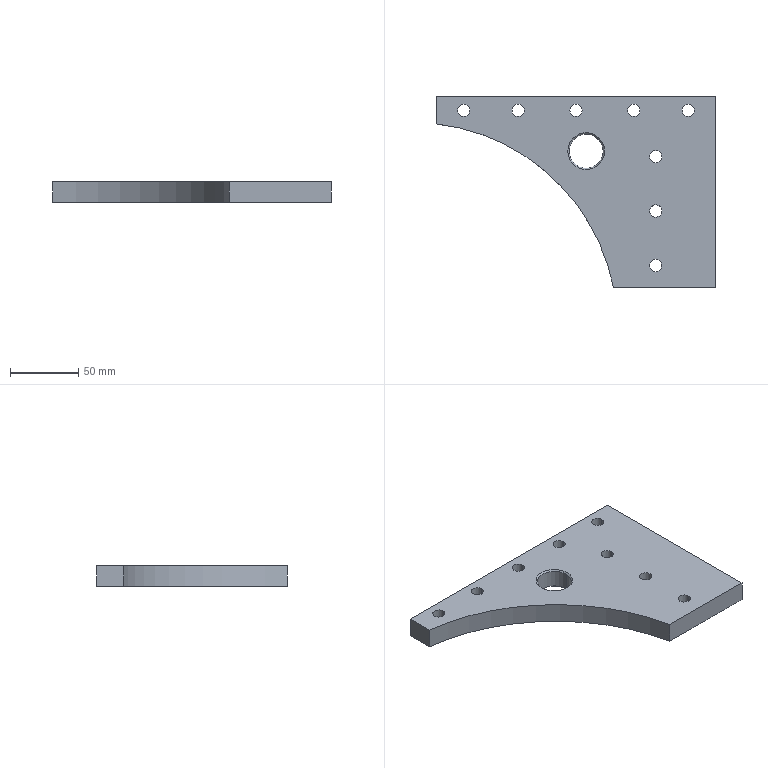Part | SolidWorks | features Cut 3, HoleWzd 2, ICE 2, Chamfer 1, Extrusion 1, Fillet 1 | 1 solid | 69 faces | box 205 x 140 x 15 mm | volume 237802 mm3 | cylinder 43 | plane 14 | cone 12 | commonest cylinder face diameters 9 x16 15 x16 4.2 x8 25 x2 300 x1